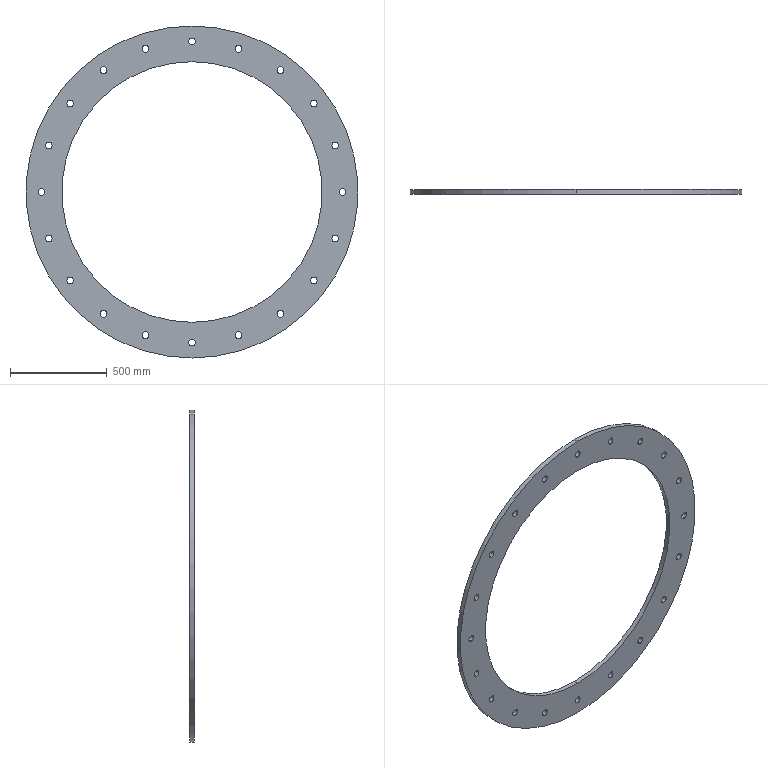Part | SolidWorks | features Extrusion 1, HoleWzd 1 | 1 solid | 46 faces | box 1720 x 25 x 1720 mm | volume 21822288 mm3 | cylinder 44 | plane 2 | commonest cylinder face diameters 35 x40 1350 x2 1720 x2